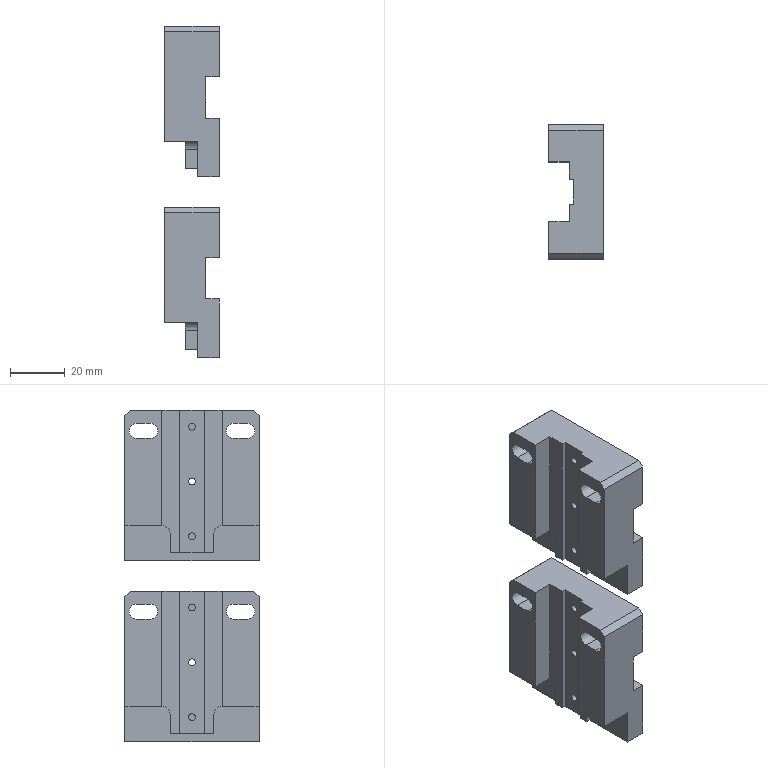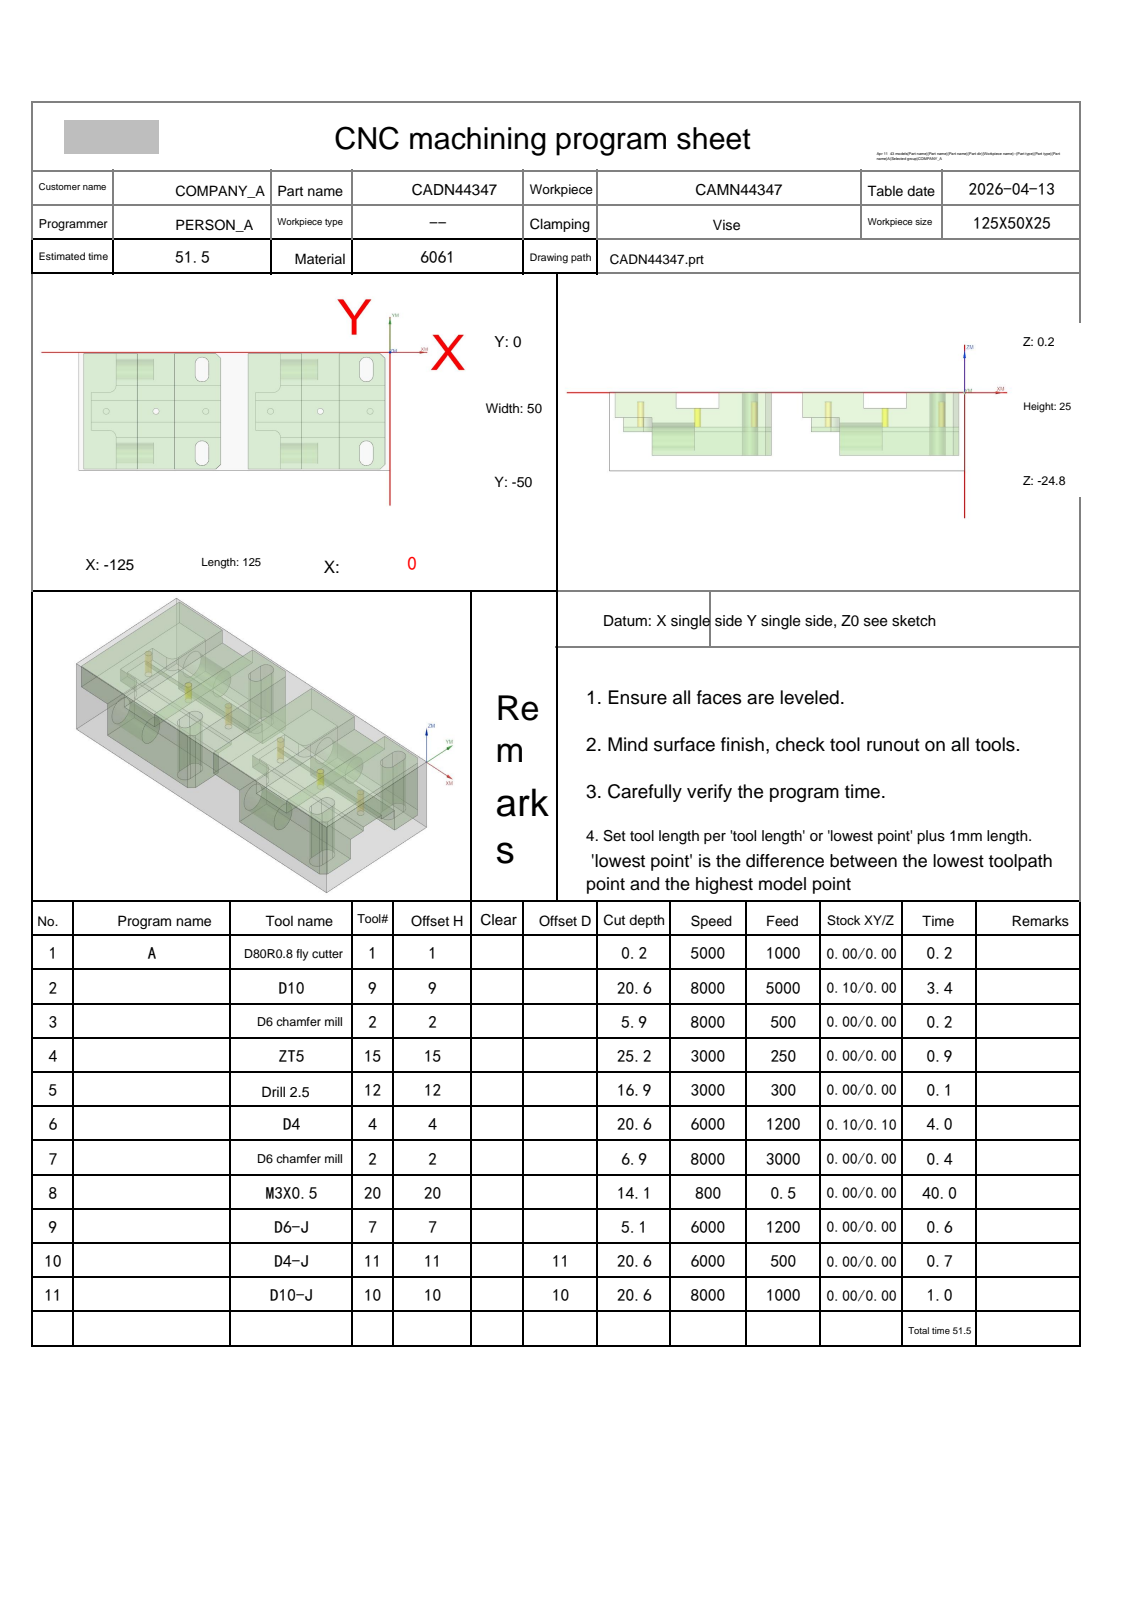NC program | NX | posted by the shop | part box 19.9 x 49 x 121 mm
Lines 1033 to 1849 of 3925:
N6 T04 M06
(D4  D=4. R=0. H=04 ce=0.10 di=0.10)
G00 G90 G54 X-10.15 Y-42.75 M03 S6000
G43 H04 Z20.
M08
Z.5
G01 Y-45.25 Z.456 F1200.
G03 X-9.5 Y-45.9 Z.438 I.65 J0.0
X-8.85 Y-45.25 Z.42 I0.0 J.65
G01 Y-40.25 Z.331
G03 X-9.5 Y-39.6 Z.313 I-.65 J0.0
X-10.15 Y-40.25 Z.295 I0.0 J-.65
G01 Y-45.25 Z.207
G03 X-9.5 Y-45.9 Z.189 I.65 J0.0
X-8.85 Y-45.25 Z.171 I0.0 J.65
G01 Y-40.25 Z.083
G03 X-9.5 Y-39.6 Z.065 I-.65 J0.0
X-10.15 Y-40.25 Z.047 I0.0 J-.65
G01 Y-45.25 Z-.042
G03 X-9.5 Y-45.9 Z-.06 I.65 J0.0
X-8.85 Y-45.25 Z-.078 I0.0 J.65
G01 Y-40.25 Z-.166
G03 X-9.5 Y-39.6 Z-.184 I-.65 J0.0
X-10.15 Y-40.25 Z-.202 I0.0 J-.65
G01 Y-45.25 Z-.291
G03 X-9.5 Y-45.9 Z-.309 I.65 J0.0
X-8.85 Y-45.25 Z-.327 I0.0 J.65
G01 Y-40.25 Z-.415
G03 X-9.5 Y-39.6 Z-.433 I-.65 J0.0
X-10.15 Y-40.25 Z-.451 I0.0 J-.65
G01 Y-45.25 Z-.539
G03 X-9.5 Y-45.9 Z-.557 I.65 J0.0
X-8.85 Y-45.25 Z-.575 I0.0 J.65
G01 Y-40.25 Z-.664
G03 X-9.5 Y-39.6 Z-.682 I-.65 J0.0
X-10.15 Y-40.25 Z-.7 I0.0 J-.65
G01 Y-45.25 Z-.788
G03 X-9.5 Y-45.9 Z-.806 I.65 J0.0
X-8.85 Y-45.25 Z-.824 I0.0 J.65
G01 Y-40.25 Z-.913
G03 X-9.5 Y-39.6 Z-.931 I-.65 J0.0
X-10.15 Y-40.25 Z-.949 I0.0 J-.65
G01 Y-45.25 Z-1.037
G03 X-9.5 Y-45.9 Z-1.055 I.65 J0.0
X-8.85 Y-45.25 Z-1.073 I0.0 J.65
G01 Y-40.25 Z-1.161
G03 X-9.5 Y-39.6 Z-1.179 I-.65 J0.0
X-10.15 Y-40.25 Z-1.198 I0.0 J-.65
G01 Y-45.25 Z-1.286
G03 X-9.5 Y-45.9 Z-1.304 I.65 J0.0
X-8.85 Y-45.25 Z-1.322 I0.0 J.65
G01 Y-40.25 Z-1.41
G03 X-9.5 Y-39.6 Z-1.428 I-.65 J0.0
X-10.15 Y-40.25 Z-1.446 I0.0 J-.65
G01 Y-45.25 Z-1.535
G03 X-9.5 Y-45.9 Z-1.553 I.65 J0.0
X-8.85 Y-45.25 Z-1.571 I0.0 J.65
G01 Y-40.25 Z-1.659
G03 X-9.5 Y-39.6 Z-1.677 I-.65 J0.0
X-10.15 Y-40.25 Z-1.695 I0.0 J-.65
G01 Y-45.25 Z-1.783
G03 X-9.5 Y-45.9 Z-1.801 I.65 J0.0
X-8.85 Y-45.25 Z-1.82 I0.0 J.65
G01 Y-40.25 Z-1.908
G03 X-9.5 Y-39.6 Z-1.926 I-.65 J0.0
X-10.15 Y-40.25 Z-1.944 I0.0 J-.65
G01 Y-45.25 Z-2.032
G03 X-9.5 Y-45.9 Z-2.05 I.65 J0.0
X-8.85 Y-45.25 Z-2.068 I0.0 J.65
G01 Y-40.25 Z-2.157
G03 X-9.5 Y-39.6 Z-2.175 I-.65 J0.0
X-10.15 Y-40.25 Z-2.193 I0.0 J-.65
G01 Y-45.25 Z-2.281
G03 X-9.5 Y-45.9 Z-2.299 I.65 J0.0
X-8.85 Y-45.25 Z-2.317 I0.0 J.65
G01 Y-40.25 Z-2.405
G03 X-9.5 Y-39.6 Z-2.424 I-.65 J0.0
X-10.15 Y-40.25 Z-2.442 I0.0 J-.65
G01 Y-45.25 Z-2.53
G03 X-9.5 Y-45.9 Z-2.548 I.65 J0.0
X-8.85 Y-45.25 Z-2.566 I0.0 J.65
G01 Y-40.25 Z-2.654
G03 X-9.5 Y-39.6 Z-2.672 I-.65 J0.0
X-10.15 Y-40.25 Z-2.69 I0.0 J-.65
G01 Y-45.25 Z-2.779
G03 X-9.5 Y-45.9 Z-2.797 I.65 J0.0
X-8.85 Y-45.25 Z-2.815 I0.0 J.65
G01 Y-40.25 Z-2.903
G03 X-9.5 Y-39.6 Z-2.921 I-.65 J0.0
X-10.15 Y-40.25 Z-2.939 I0.0 J-.65
G01 Y-45.25 Z-3.027
G03 X-9.5 Y-45.9 Z-3.046 I.65 J0.0
X-8.85 Y-45.25 Z-3.064 I0.0 J.65
G01 Y-40.25 Z-3.152
G03 X-9.5 Y-39.6 Z-3.17 I-.65 J0.0
X-10.15 Y-40.25 Z-3.188 I0.0 J-.65
G01 Y-45.25 Z-3.276
G03 X-9.5 Y-45.9 Z-3.294 I.65 J0.0
X-8.85 Y-45.25 Z-3.312 I0.0 J.65
G01 Y-40.25 Z-3.401
G03 X-9.5 Y-39.6 Z-3.419 I-.65 J0.0
X-10.15 Y-40.25 Z-3.437 I0.0 J-.65
G01 Y-45.25 Z-3.525
G03 X-9.5 Y-45.9 Z-3.543 I.65 J0.0
X-8.85 Y-45.25 Z-3.561 I0.0 J.65
G01 Y-40.25 Z-3.65
G03 X-9.5 Y-39.6 Z-3.668 I-.65 J0.0
X-10.15 Y-40.25 Z-3.686 I0.0 J-.65
G01 Y-45.25 Z-3.774
G03 X-9.5 Y-45.9 Z-3.792 I.65 J0.0
X-8.85 Y-45.25 Z-3.81 I0.0 J.65
G01 Y-40.25 Z-3.898
G03 X-9.5 Y-39.6 Z-3.916 I-.65 J0.0
X-10.15 Y-40.25 Z-3.934 I0.0 J-.65
G01 Y-45.25 Z-4.023
G03 X-9.5 Y-45.9 Z-4.041 I.65 J0.0
X-8.85 Y-45.25 Z-4.059 I0.0 J.65
G01 Y-40.25 Z-4.147
G03 X-9.5 Y-39.6 Z-4.165 I-.65 J0.0
X-10.15 Y-40.25 Z-4.183 I0.0 J-.65
G01 Y-45.25 Z-4.272
G03 X-9.5 Y-45.9 Z-4.29 I.65 J0.0
X-8.85 Y-45.25 Z-4.308 I0.0 J.65
G01 Y-40.25 Z-4.396
G03 X-9.5 Y-39.6 Z-4.414 I-.65 J0.0
X-10.15 Y-40.25 Z-4.432 I0.0 J-.65
G01 Y-45.25 Z-4.52
G03 X-9.5 Y-45.9 Z-4.538 I.65 J0.0
X-8.85 Y-45.25 Z-4.556 I0.0 J.65
G01 Y-40.25 Z-4.645
G03 X-9.5 Y-39.6 Z-4.663 I-.65 J0.0
X-10.15 Y-40.25 Z-4.681 I0.0 J-.65
G01 Y-45.25 Z-4.769
G03 X-9.5 Y-45.9 Z-4.787 I.65 J0.0
X-8.85 Y-45.25 Z-4.805 I0.0 J.65
G01 Y-40.25 Z-4.894
G03 X-9.5 Y-39.6 Z-4.912 I-.65 J0.0
X-10.15 Y-40.25 Z-4.93 I0.0 J-.65
G01 Y-45.25 Z-5.018
G03 X-9.5 Y-45.9 Z-5.036 I.65 J0.0
X-8.85 Y-45.25 Z-5.054 I0.0 J.65
G01 Y-40.25 Z-5.142
G03 X-9.5 Y-39.6 Z-5.16 I-.65 J0.0
X-10.15 Y-40.25 Z-5.178 I0.0 J-.65
G01 Y-45.25 Z-5.267
G03 X-9.5 Y-45.9 Z-5.285 I.65 J0.0
X-8.85 Y-45.25 Z-5.303 I0.0 J.65
G01 Y-40.25 Z-5.391
G03 X-9.5 Y-39.6 Z-5.409 I-.65 J0.0
X-10.15 Y-40.25 Z-5.427 I0.0 J-.65
G01 Y-45.25 Z-5.516
G03 X-9.5 Y-45.9 Z-5.534 I.65 J0.0
X-8.85 Y-45.25 Z-5.552 I0.0 J.65
G01 Y-40.25 Z-5.64
G03 X-9.5 Y-39.6 Z-5.658 I-.65 J0.0
X-10.15 Y-40.25 Z-5.676 I0.0 J-.65
G01 Y-45.25 Z-5.764
G03 X-9.5 Y-45.9 Z-5.782 I.65 J0.0
X-8.85 Y-45.25 Z-5.8 I0.0 J.65
G01 Y-40.25 Z-5.889
G03 X-9.5 Y-39.6 Z-5.907 I-.65 J0.0
X-10.15 Y-40.25 Z-5.925 I0.0 J-.65
G01 Y-45.25 Z-6.013
G03 X-9.5 Y-45.9 Z-6.031 I.65 J0.0
X-8.85 Y-45.25 Z-6.049 I0.0 J.65
G01 Y-40.25 Z-6.138
G03 X-9.5 Y-39.6 Z-6.156 I-.65 J0.0
X-10.15 Y-40.25 Z-6.174 I0.0 J-.65
G01 Y-45.25 Z-6.262
G03 X-9.5 Y-45.9 Z-6.28 I.65 J0.0
X-8.85 Y-45.25 Z-6.298 I0.0 J.65
G01 Y-40.25 Z-6.386
G03 X-9.5 Y-39.6 Z-6.404 I-.65 J0.0
X-10.15 Y-40.25 Z-6.423 I0.0 J-.65
G01 Y-45.25 Z-6.511
G03 X-9.5 Y-45.9 Z-6.529 I.65 J0.0
X-8.85 Y-45.25 Z-6.547 I0.0 J.65
G01 Y-40.25 Z-6.635
G03 X-9.5 Y-39.6 Z-6.653 I-.65 J0.0
X-10.15 Y-40.25 Z-6.671 I0.0 J-.65
G01 Y-45.25 Z-6.76
G03 X-9.5 Y-45.9 Z-6.778 I.65 J0.0
X-8.85 Y-45.25 Z-6.796 I0.0 J.65
G01 Y-40.25 Z-6.884
G03 X-9.5 Y-39.6 Z-6.902 I-.65 J0.0
X-10.15 Y-40.25 Z-6.92 I0.0 J-.65
G01 Y-45.25 Z-7.008
G03 X-9.5 Y-45.9 Z-7.026 I.65 J0.0
X-8.85 Y-45.25 Z-7.045 I0.0 J.65
G01 Y-40.25 Z-7.133
G03 X-9.5 Y-39.6 Z-7.151 I-.65 J0.0
X-10.15 Y-40.25 Z-7.169 I0.0 J-.65
G01 Y-45.25 Z-7.257
G03 X-9.5 Y-45.9 Z-7.275 I.65 J0.0
X-8.85 Y-45.25 Z-7.293 I0.0 J.65
G01 Y-40.25 Z-7.382
G03 X-9.5 Y-39.6 Z-7.4 I-.65 J0.0
X-10.15 Y-40.25 Z-7.418 I0.0 J-.65
G01 Y-45.25 Z-7.506
G03 X-9.5 Y-45.9 Z-7.524 I.65 J0.0
X-8.85 Y-45.25 Z-7.542 I0.0 J.65
G01 Y-40.25 Z-7.63
G03 X-9.5 Y-39.6 Z-7.649 I-.65 J0.0
X-10.15 Y-40.25 Z-7.667 I0.0 J-.65
G01 Y-45.25 Z-7.755
G03 X-9.5 Y-45.9 Z-7.773 I.65 J0.0
X-8.85 Y-45.25 Z-7.791 I0.0 J.65
G01 Y-40.25 Z-7.879
G03 X-9.5 Y-39.6 Z-7.897 I-.65 J0.0
X-10.15 Y-40.25 Z-7.915 I0.0 J-.65
G01 Y-45.25 Z-8.004
G03 X-9.5 Y-45.9 Z-8.022 I.65 J0.0
X-8.85 Y-45.25 Z-8.04 I0.0 J.65
G01 Y-40.25 Z-8.128
G03 X-9.5 Y-39.6 Z-8.146 I-.65 J0.0
X-10.15 Y-40.25 Z-8.164 I0.0 J-.65
G01 Y-45.25 Z-8.252
G03 X-9.5 Y-45.9 Z-8.271 I.65 J0.0
X-8.85 Y-45.25 Z-8.289 I0.0 J.65
G01 Y-40.25 Z-8.377
G03 X-9.5 Y-39.6 Z-8.395 I-.65 J0.0
X-10.15 Y-40.25 Z-8.413 I0.0 J-.65
G01 Y-45.25 Z-8.501
G03 X-9.5 Y-45.9 Z-8.519 I.65 J0.0
X-8.85 Y-45.25 Z-8.537 I0.0 J.65
G01 Y-40.25 Z-8.626
G03 X-9.5 Y-39.6 Z-8.644 I-.65 J0.0
X-10.15 Y-40.25 Z-8.662 I0.0 J-.65
G01 Y-45.25 Z-8.75
G03 X-9.5 Y-45.9 Z-8.768 I.65 J0.0
X-8.85 Y-45.25 Z-8.786 I0.0 J.65
G01 Y-40.25 Z-8.875
G03 X-9.5 Y-39.6 Z-8.893 I-.65 J0.0
X-10.15 Y-40.25 Z-8.911 I0.0 J-.65
G01 Y-45.25 Z-8.999
G03 X-9.5 Y-45.9 Z-9.017 I.65 J0.0
X-8.85 Y-45.25 Z-9.035 I0.0 J.65
G01 Y-40.25 Z-9.123
G03 X-9.5 Y-39.6 Z-9.141 I-.65 J0.0
X-10.15 Y-40.25 Z-9.159 I0.0 J-.65
G01 Y-45.25 Z-9.248
G03 X-9.5 Y-45.9 Z-9.266 I.65 J0.0
X-8.85 Y-45.25 Z-9.284 I0.0 J.65
G01 Y-40.25 Z-9.372
G03 X-9.5 Y-39.6 Z-9.39 I-.65 J0.0
X-10.15 Y-40.25 Z-9.408 I0.0 J-.65
G01 Y-45.25 Z-9.497
G03 X-9.5 Y-45.9 Z-9.515 I.65 J0.0
X-8.85 Y-45.25 Z-9.533 I0.0 J.65
G01 Y-40.25 Z-9.621
G03 X-9.5 Y-39.6 Z-9.639 I-.65 J0.0
X-10.15 Y-40.25 Z-9.657 I0.0 J-.65
G01 Y-45.25 Z-9.745
G03 X-9.5 Y-45.9 Z-9.763 I.65 J0.0
X-8.85 Y-45.25 Z-9.781 I0.0 J.65
G01 Y-40.25 Z-9.87
G03 X-9.5 Y-39.6 Z-9.888 I-.65 J0.0
X-10.15 Y-40.25 Z-9.906 I0.0 J-.65
G01 Y-45.25 Z-9.994
G03 X-9.5 Y-45.9 Z-10.012 I.65 J0.0
X-8.85 Y-45.25 Z-10.03 I0.0 J.65
G01 Y-40.25 Z-10.119
G03 X-9.5 Y-39.6 Z-10.137 I-.65 J0.0
X-10.15 Y-40.25 Z-10.155 I0.0 J-.65
G01 Y-45.25 Z-10.243
G03 X-9.5 Y-45.9 Z-10.261 I.65 J0.0
X-8.85 Y-45.25 Z-10.279 I0.0 J.65
G01 Y-40.25 Z-10.367
G03 X-9.5 Y-39.6 Z-10.385 I-.65 J0.0
X-10.15 Y-40.25 Z-10.403 I0.0 J-.65
G01 Y-45.25 Z-10.492
G03 X-9.5 Y-45.9 Z-10.51 I.65 J0.0
X-8.85 Y-45.25 Z-10.528 I0.0 J.65
G01 Y-40.25 Z-10.616
G03 X-9.5 Y-39.6 Z-10.634 I-.65 J0.0
X-10.15 Y-40.25 Z-10.652 I0.0 J-.65
G01 Y-45.25 Z-10.741
G03 X-9.5 Y-45.9 Z-10.759 I.65 J0.0
X-8.85 Y-45.25 Z-10.777 I0.0 J.65
G01 Y-40.25 Z-10.865
G03 X-9.5 Y-39.6 Z-10.883 I-.65 J0.0
X-10.15 Y-40.25 Z-10.901 I0.0 J-.65
G01 Y-45.25 Z-10.989
G03 X-9.5 Y-45.9 Z-11.007 I.65 J0.0
X-8.85 Y-45.25 Z-11.025 I0.0 J.65
G01 Y-40.25 Z-11.114
G03 X-9.5 Y-39.6 Z-11.132 I-.65 J0.0
X-10.15 Y-40.25 Z-11.15 I0.0 J-.65
G01 Y-45.25 Z-11.238
G03 X-9.5 Y-45.9 Z-11.256 I.65 J0.0
X-8.85 Y-45.25 Z-11.274 I0.0 J.65
G01 Y-40.25 Z-11.363
G03 X-9.5 Y-39.6 Z-11.381 I-.65 J0.0
X-10.15 Y-40.25 Z-11.399 I0.0 J-.65
G01 Y-45.25 Z-11.487
G03 X-9.5 Y-45.9 Z-11.505 I.65 J0.0
X-8.85 Y-45.25 Z-11.523 I0.0 J.65
G01 Y-40.25 Z-11.611
G03 X-9.5 Y-39.6 Z-11.629 I-.65 J0.0
X-10.15 Y-40.25 Z-11.648 I0.0 J-.65
G01 Y-45.25 Z-11.736
G03 X-9.5 Y-45.9 Z-11.754 I.65 J0.0
X-8.85 Y-45.25 Z-11.772 I0.0 J.65
G01 Y-40.25 Z-11.86
G03 X-9.5 Y-39.6 Z-11.878 I-.65 J0.0
X-10.15 Y-40.25 Z-11.896 I0.0 J-.65
G01 Y-45.25 Z-11.985
G03 X-9.5 Y-45.9 Z-12.003 I.65 J0.0
X-8.85 Y-45.25 Z-12.021 I0.0 J.65
G01 Y-40.25 Z-12.109
G03 X-9.5 Y-39.6 Z-12.127 I-.65 J0.0
X-10.15 Y-40.25 Z-12.145 I0.0 J-.65
G01 Y-45.25 Z-12.233
G03 X-9.5 Y-45.9 Z-12.251 I.65 J0.0
X-8.85 Y-45.25 Z-12.27 I0.0 J.65
G01 Y-40.25 Z-12.358
G03 X-9.5 Y-39.6 Z-12.376 I-.65 J0.0
X-10.15 Y-40.25 Z-12.394 I0.0 J-.65
G01 Y-45.25 Z-12.482
G03 X-9.5 Y-45.9 Z-12.5 I.65 J0.0
X-8.85 Y-45.25 Z-12.518 I0.0 J.65
G01 Y-40.25 Z-12.607
G03 X-9.5 Y-39.6 Z-12.625 I-.65 J0.0
X-10.15 Y-40.25 Z-12.643 I0.0 J-.65
G01 Y-45.25 Z-12.731
G03 X-9.5 Y-45.9 Z-12.749 I.65 J0.0
X-8.85 Y-45.25 Z-12.767 I0.0 J.65
G01 Y-40.25 Z-12.855
G03 X-9.5 Y-39.6 Z-12.874 I-.65 J0.0
X-10.15 Y-40.25 Z-12.892 I0.0 J-.65
G01 Y-45.25 Z-12.98
G03 X-9.5 Y-45.9 Z-12.998 I.65 J0.0
X-8.85 Y-45.25 Z-13.016 I0.0 J.65
G01 Y-40.25 Z-13.104
G03 X-9.5 Y-39.6 Z-13.122 I-.65 J0.0
X-10.15 Y-40.25 Z-13.14 I0.0 J-.65
G01 Y-45.25 Z-13.229
G03 X-9.5 Y-45.9 Z-13.247 I.65 J0.0
X-8.85 Y-45.25 Z-13.265 I0.0 J.65
G01 Y-40.25 Z-13.353
G03 X-9.5 Y-39.6 Z-13.371 I-.65 J0.0
X-10.15 Y-40.25 Z-13.389 I0.0 J-.65
G01 Y-45.25 Z-13.477
G03 X-9.5 Y-45.9 Z-13.496 I.65 J0.0
X-8.85 Y-45.25 Z-13.514 I0.0 J.65
G01 Y-40.25 Z-13.602
G03 X-9.5 Y-39.6 Z-13.62 I-.65 J0.0
X-10.15 Y-40.25 Z-13.638 I0.0 J-.65
G01 Y-45.25 Z-13.726
G03 X-9.5 Y-45.9 Z-13.744 I.65 J0.0
X-8.85 Y-45.25 Z-13.762 I0.0 J.65
G01 Y-40.25 Z-13.851
G03 X-9.5 Y-39.6 Z-13.869 I-.65 J0.0
X-10.15 Y-40.25 Z-13.887 I0.0 J-.65
G01 Y-45.25 Z-13.975
G03 X-9.5 Y-45.9 Z-13.993 I.65 J0.0
X-8.85 Y-45.25 Z-14.011 I0.0 J.65
G01 Y-40.25 Z-14.1
G03 X-9.5 Y-39.6 Z-14.118 I-.65 J0.0
X-10.15 Y-40.25 Z-14.136 I0.0 J-.65
G01 Y-45.25 Z-14.224
G03 X-9.5 Y-45.9 Z-14.242 I.65 J0.0
X-8.85 Y-45.25 Z-14.26 I0.0 J.65
G01 Y-40.25 Z-14.348
G03 X-9.5 Y-39.6 Z-14.366 I-.65 J0.0
X-10.15 Y-40.25 Z-14.384 I0.0 J-.65
G01 Y-45.25 Z-14.473
G03 X-9.5 Y-45.9 Z-14.491 I.65 J0.0
X-8.85 Y-45.25 Z-14.509 I0.0 J.65
G01 Y-40.25 Z-14.597
G03 X-9.5 Y-39.6 Z-14.615 I-.65 J0.0
X-10.15 Y-40.25 Z-14.633 I0.0 J-.65
G01 Y-45.25 Z-14.722
G03 X-9.5 Y-45.9 Z-14.74 I.65 J0.0
X-8.85 Y-45.25 Z-14.758 I0.0 J.65
G01 Y-40.25 Z-14.846
G03 X-9.5 Y-39.6 Z-14.864 I-.65 J0.0
X-10.15 Y-40.25 Z-14.882 I0.0 J-.65
G01 Y-45.25 Z-14.97
G03 X-9.5 Y-45.9 Z-14.988 I.65 J0.0
X-8.85 Y-45.25 Z-15.006 I0.0 J.65
G01 Y-40.25 Z-15.095
G03 X-9.5 Y-39.6 Z-15.113 I-.65 J0.0
X-10.15 Y-40.25 Z-15.131 I0.0 J-.65
G01 Y-45.25 Z-15.219
G03 X-9.5 Y-45.9 Z-15.237 I.65 J0.0
X-8.85 Y-45.25 Z-15.255 I0.0 J.65
G01 Y-40.25 Z-15.344
G03 X-9.5 Y-39.6 Z-15.362 I-.65 J0.0
X-10.15 Y-40.25 Z-15.38 I0.0 J-.65
G01 Y-45.25 Z-15.468
G03 X-9.5 Y-45.9 Z-15.486 I.65 J0.0
X-8.85 Y-45.25 Z-15.504 I0.0 J.65
G01 Y-40.25 Z-15.592
G03 X-9.5 Y-39.6 Z-15.61 I-.65 J0.0
X-10.15 Y-40.25 Z-15.628 I0.0 J-.65
G01 Y-45.25 Z-15.717
G03 X-9.5 Y-45.9 Z-15.735 I.65 J0.0
X-8.85 Y-45.25 Z-15.753 I0.0 J.65
G01 Y-40.25 Z-15.841
G03 X-9.5 Y-39.6 Z-15.859 I-.65 J0.0
X-10.15 Y-40.25 Z-15.877 I0.0 J-.65
G01 Y-45.25 Z-15.966
G03 X-9.5 Y-45.9 Z-15.984 I.65 J0.0
X-8.85 Y-45.25 Z-16.002 I0.0 J.65
G01 Y-40.25 Z-16.09
G03 X-9.5 Y-39.6 Z-16.108 I-.65 J0.0
X-10.15 Y-40.25 Z-16.126 I0.0 J-.65
G01 Y-45.25 Z-16.214
G03 X-9.5 Y-45.9 Z-16.232 I.65 J0.0
X-8.85 Y-45.25 Z-16.25 I0.0 J.65
G01 Y-40.25 Z-16.339
G03 X-9.5 Y-39.6 Z-16.357 I-.65 J0.0
X-10.15 Y-40.25 Z-16.375 I0.0 J-.65
G01 Y-45.25 Z-16.463
G03 X-9.5 Y-45.9 Z-16.481 I.65 J0.0
X-8.85 Y-45.25 Z-16.499 I0.0 J.65
G01 Y-40.25 Z-16.588
G03 X-9.5 Y-39.6 Z-16.606 I-.65 J0.0
X-10.15 Y-40.25 Z-16.624 I0.0 J-.65
G01 Y-45.25 Z-16.712
G03 X-9.5 Y-45.9 Z-16.73 I.65 J0.0
X-8.85 Y-45.25 Z-16.748 I0.0 J.65
G01 Y-40.25 Z-16.836
G03 X-9.5 Y-39.6 Z-16.854 I-.65 J0.0
X-10.15 Y-40.25 Z-16.873 I0.0 J-.65
G01 Y-45.25 Z-16.961
G03 X-9.5 Y-45.9 Z-16.979 I.65 J0.0
X-8.85 Y-45.25 Z-16.997 I0.0 J.65
G01 Y-40.25 Z-17.085
G03 X-9.5 Y-39.6 Z-17.103 I-.65 J0.0
X-10.15 Y-40.25 Z-17.121 I0.0 J-.65
G01 Y-45.25 Z-17.21
G03 X-9.5 Y-45.9 Z-17.228 I.65 J0.0
X-8.85 Y-45.25 Z-17.246 I0.0 J.65
G01 Y-40.25 Z-17.334
G03 X-9.5 Y-39.6 Z-17.352 I-.65 J0.0
X-10.15 Y-40.25 Z-17.37 I0.0 J-.65
G01 Y-45.25 Z-17.458
G03 X-9.5 Y-45.9 Z-17.476 I.65 J0.0
X-8.85 Y-45.25 Z-17.495 I0.0 J.65
G01 Y-40.25 Z-17.583
G03 X-9.5 Y-39.6 Z-17.601 I-.65 J0.0
X-10.15 Y-40.25 Z-17.619 I0.0 J-.65
G01 Y-45.25 Z-17.707
G03 X-9.5 Y-45.9 Z-17.725 I.65 J0.0
X-8.85 Y-45.25 Z-17.743 I0.0 J.65
G01 Y-40.25 Z-17.832
G03 X-9.5 Y-39.6 Z-17.85 I-.65 J0.0
X-10.15 Y-40.25 Z-17.868 I0.0 J-.65
G01 Y-45.25 Z-17.956
G03 X-9.5 Y-45.9 Z-17.974 I.65 J0.0
X-8.85 Y-45.25 Z-17.992 I0.0 J.65
G01 Y-40.25 Z-18.08
G03 X-9.5 Y-39.6 Z-18.099 I-.65 J0.0
X-10.15 Y-40.25 Z-18.117 I0.0 J-.65
G01 Y-45.25 Z-18.205
G03 X-9.5 Y-45.9 Z-18.223 I.65 J0.0
X-8.85 Y-45.25 Z-18.241 I0.0 J.65
G01 Y-40.25 Z-18.329
G03 X-9.5 Y-39.6 Z-18.347 I-.65 J0.0
X-10.15 Y-40.25 Z-18.365 I0.0 J-.65
G01 Y-45.25 Z-18.454
G03 X-9.5 Y-45.9 Z-18.472 I.65 J0.0
X-8.85 Y-45.25 Z-18.49 I0.0 J.65
G01 Y-40.25 Z-18.578
G03 X-9.5 Y-39.6 Z-18.596 I-.65 J0.0
X-10.15 Y-40.25 Z-18.614 I0.0 J-.65
G01 Y-45.25 Z-18.702
G03 X-9.5 Y-45.9 Z-18.721 I.65 J0.0
X-8.85 Y-45.25 Z-18.739 I0.0 J.65
G01 Y-40.25 Z-18.827
G03 X-9.5 Y-39.6 Z-18.845 I-.65 J0.0
X-10.15 Y-40.25 Z-18.863 I0.0 J-.65
G01 Y-45.25 Z-18.951
G03 X-9.5 Y-45.9 Z-18.969 I.65 J0.0
X-8.85 Y-45.25 Z-18.987 I0.0 J.65
G01 Y-40.25 Z-19.076
G03 X-9.5 Y-39.6 Z-19.094 I-.65 J0.0
X-10.15 Y-40.25 Z-19.112 I0.0 J-.65
G01 Y-45.25 Z-19.2
G03 X-9.5 Y-45.9 Z-19.218 I.65 J0.0
X-8.85 Y-45.25 Z-19.236 I0.0 J.65
G01 Y-40.25 Z-19.325
G03 X-9.5 Y-39.6 Z-19.343 I-.65 J0.0
X-10.15 Y-40.25 Z-19.361 I0.0 J-.65
G01 Y-45.25 Z-19.449
G03 X-9.5 Y-45.9 Z-19.467 I.65 J0.0
X-8.85 Y-45.25 Z-19.485 I0.0 J.65
G01 Y-40.25 Z-19.573
G03 X-9.5 Y-39.6 Z-19.591 I-.65 J0.0
X-10.15 Y-40.25 Z-19.609 I0.0 J-.65
G01 Y-45.25 Z-19.698
G03 X-9.5 Y-45.9 Z-19.716 I.65 J0.0
X-8.85 Y-45.25 Z-19.734 I0.0 J.65
G01 Y-40.25 Z-19.822
G03 X-9.5 Y-39.6 Z-19.84 I-.65 J0.0
X-10.15 Y-40.25 Z-19.858 I0.0 J-.65
G01 Y-45.25 Z-19.947
G03 X-9.5 Y-45.9 Z-19.965 I.65 J0.0
X-8.85 Y-45.25 Z-19.983 I0.0 J.65
G01 Y-40.25 Z-20.071
G03 X-9.5 Y-39.6 Z-20.089 I-.65 J0.0
X-10.15 Y-40.25 Z-20.107 I0.0 J-.65
G01 Y-45.25 Z-20.195
G03 X-9.5 Y-45.9 Z-20.213 I.65 J0.0
X-8.85 Y-45.25 Z-20.231 I0.0 J.65
G01 Y-40.25 Z-20.32
G03 X-9.5 Y-39.6 Z-20.338 I-.65 J0.0
X-10.15 Y-40.25 Z-20.356 I0.0 J-.65
G01 Y-42.75 Z-20.4
Y-45.25
G03 X-9.5 Y-45.9 I.65 J0.0
X-8.85 Y-45.25 I0.0 J.65
G01 Y-40.25
G03 X-9.5 Y-39.6 I-.65 J0.0
X-10.15 Y-40.25 I0.0 J-.65
G01 Y-42.75
Y-43.25
Z-19.4
G00 Z20.
X-8.85 Y-7.25
Z.5
G01 Y-4.75 Z.456
G03 X-9.5 Y-4.1 Z.438 I-.65 J0.0
X-10.15 Y-4.75 Z.42 I0.0 J-.65
G01 Y-9.75 Z.331
G03 X-9.5 Y-10.4 Z.313 I.65 J0.0
X-8.85 Y-9.75 Z.295 I0.0 J.65
G01 Y-4.75 Z.207
G03 X-9.5 Y-4.1 Z.189 I-.65 J0.0
X-10.15 Y-4.75 Z.171 I0.0 J-.65
G01 Y-9.75 Z.083
G03 X-9.5 Y-10.4 Z.065 I.65 J0.0
X-8.85 Y-9.75 Z.047 I0.0 J.65
G01 Y-4.75 Z-.042
G03 X-9.5 Y-4.1 Z-.06 I-.65 J0.0
X-10.15 Y-4.75 Z-.078 I0.0 J-.65
G01 Y-9.75 Z-.166
G03 X-9.5 Y-10.4 Z-.184 I.65 J0.0
X-8.85 Y-9.75 Z-.202 I0.0 J.65
G01 Y-4.75 Z-.291
G03 X-9.5 Y-4.1 Z-.309 I-.65 J0.0
X-10.15 Y-4.75 Z-.327 I0.0 J-.65
G01 Y-9.75 Z-.415
G03 X-9.5 Y-10.4 Z-.433 I.65 J0.0
X-8.85 Y-9.75 Z-.451 I0.0 J.65
G01 Y-4.75 Z-.539
G03 X-9.5 Y-4.1 Z-.557 I-.65 J0.0
X-10.15 Y-4.75 Z-.575 I0.0 J-.65
G01 Y-9.75 Z-.664
G03 X-9.5 Y-10.4 Z-.682 I.65 J0.0
X-8.85 Y-9.75 Z-.7 I0.0 J.65
G01 Y-4.75 Z-.788
G03 X-9.5 Y-4.1 Z-.806 I-.65 J0.0
X-10.15 Y-4.75 Z-.824 I0.0 J-.65
G01 Y-9.75 Z-.913
G03 X-9.5 Y-10.4 Z-.931 I.65 J0.0
X-8.85 Y-9.75 Z-.949 I0.0 J.65
G01 Y-4.75 Z-1.037
G03 X-9.5 Y-4.1 Z-1.055 I-.65 J0.0
X-10.15 Y-4.75 Z-1.073 I0.0 J-.65
G01 Y-9.75 Z-1.161
G03 X-9.5 Y-10.4 Z-1.179 I.65 J0.0
X-8.85 Y-9.75 Z-1.198 I0.0 J.65
G01 Y-4.75 Z-1.286
G03 X-9.5 Y-4.1 Z-1.304 I-.65 J0.0
X-10.15 Y-4.75 Z-1.322 I0.0 J-.65
G01 Y-9.75 Z-1.41
G03 X-9.5 Y-10.4 Z-1.428 I.65 J0.0
X-8.85 Y-9.75 Z-1.446 I0.0 J.65
G01 Y-4.75 Z-1.535
G03 X-9.5 Y-4.1 Z-1.553 I-.65 J0.0
X-10.15 Y-4.75 Z-1.571 I0.0 J-.65
G01 Y-9.75 Z-1.659
G03 X-9.5 Y-10.4 Z-1.677 I.65 J0.0
X-8.85 Y-9.75 Z-1.695 I0.0 J.65
G01 Y-4.75 Z-1.783
G03 X-9.5 Y-4.1 Z-1.801 I-.65 J0.0
X-10.15 Y-4.75 Z-1.82 I0.0 J-.65
G01 Y-9.75 Z-1.908
G03 X-9.5 Y-10.4 Z-1.926 I.65 J0.0
X-8.85 Y-9.75 Z-1.944 I0.0 J.65
G01 Y-4.75 Z-2.032
G03 X-9.5 Y-4.1 Z-2.05 I-.65 J0.0
X-10.15 Y-4.75 Z-2.068 I0.0 J-.65
G01 Y-9.75 Z-2.157
G03 X-9.5 Y-10.4 Z-2.175 I.65 J0.0
X-8.85 Y-9.75 Z-2.193 I0.0 J.65
G01 Y-4.75 Z-2.281
G03 X-9.5 Y-4.1 Z-2.299 I-.65 J0.0
X-10.15 Y-4.75 Z-2.317 I0.0 J-.65
G01 Y-9.75 Z-2.405
G03 X-9.5 Y-10.4 Z-2.424 I.65 J0.0
X-8.85 Y-9.75 Z-2.442 I0.0 J.65
G01 Y-4.75 Z-2.53
G03 X-9.5 Y-4.1 Z-2.548 I-.65 J0.0
X-10.15 Y-4.75 Z-2.566 I0.0 J-.65
G01 Y-9.75 Z-2.654
G03 X-9.5 Y-10.4 Z-2.672 I.65 J0.0
X-8.85 Y-9.75 Z-2.69 I0.0 J.65
G01 Y-4.75 Z-2.779
G03 X-9.5 Y-4.1 Z-2.797 I-.65 J0.0
X-10.15 Y-4.75 Z-2.815 I0.0 J-.65
G01 Y-9.75 Z-2.903
G03 X-9.5 Y-10.4 Z-2.921 I.65 J0.0
X-8.85 Y-9.75 Z-2.939 I0.0 J.65
G01 Y-4.75 Z-3.027
G03 X-9.5 Y-4.1 Z-3.046 I-.65 J0.0
X-10.15 Y-4.75 Z-3.064 I0.0 J-.65
G01 Y-9.75 Z-3.152
G03 X-9.5 Y-10.4 Z-3.17 I.65 J0.0
X-8.85 Y-9.75 Z-3.188 I0.0 J.65
G01 Y-4.75 Z-3.276
G03 X-9.5 Y-4.1 Z-3.294 I-.65 J0.0
X-10.15 Y-4.75 Z-3.312 I0.0 J-.65
G01 Y-9.75 Z-3.401
G03 X-9.5 Y-10.4 Z-3.419 I.65 J0.0
X-8.85 Y-9.75 Z-3.437 I0.0 J.65
G01 Y-4.75 Z-3.525
G03 X-9.5 Y-4.1 Z-3.543 I-.65 J0.0
X-10.15 Y-4.75 Z-3.561 I0.0 J-.65
G01 Y-9.75 Z-3.65
G03 X-9.5 Y-10.4 Z-3.668 I.65 J0.0
X-8.85 Y-9.75 Z-3.686 I0.0 J.65
G01 Y-4.75 Z-3.774
G03 X-9.5 Y-4.1 Z-3.792 I-.65 J0.0
X-10.15 Y-4.75 Z-3.81 I0.0 J-.65
G01 Y-9.75 Z-3.898
G03 X-9.5 Y-10.4 Z-3.916 I.65 J0.0
X-8.85 Y-9.75 Z-3.934 I0.0 J.65
G01 Y-4.75 Z-4.023
G03 X-9.5 Y-4.1 Z-4.041 I-.65 J0.0
X-10.15 Y-4.75 Z-4.059 I0.0 J-.65
G01 Y-9.75 Z-4.147
G03 X-9.5 Y-10.4 Z-4.165 I.65 J0.0
X-8.85 Y-9.75 Z-4.183 I0.0 J.65
G01 Y-4.75 Z-4.272
G03 X-9.5 Y-4.1 Z-4.29 I-.65 J0.0
X-10.15 Y-4.75 Z-4.308 I0.0 J-.65
G01 Y-9.75 Z-4.396
G03 X-9.5 Y-10.4 Z-4.414 I.65 J0.0
X-8.85 Y-9.75 Z-4.432 I0.0 J.65
G01 Y-4.75 Z-4.52
G03 X-9.5 Y-4.1 Z-4.538 I-.65 J0.0
X-10.15 Y-4.75 Z-4.556 I0.0 J-.65
G01 Y-9.75 Z-4.645
G03 X-9.5 Y-10.4 Z-4.663 I.65 J0.0
X-8.85 Y-9.75 Z-4.681 I0.0 J.65
G01 Y-4.75 Z-4.769
G03 X-9.5 Y-4.1 Z-4.787 I-.65 J0.0
X-10.15 Y-4.75 Z-4.805 I0.0 J-.65
G01 Y-9.75 Z-4.894
G03 X-9.5 Y-10.4 Z-4.912 I.65 J0.0
X-8.85 Y-9.75 Z-4.93 I0.0 J.65
G01 Y-4.75 Z-5.018
G03 X-9.5 Y-4.1 Z-5.036 I-.65 J0.0
X-10.15 Y-4.75 Z-5.054 I0.0 J-.65
G01 Y-9.75 Z-5.142
G03 X-9.5 Y-10.4 Z-5.16 I.65 J0.0
X-8.85 Y-9.75 Z-5.178 I0.0 J.65
G01 Y-4.75 Z-5.267
G03 X-9.5 Y-4.1 Z-5.285 I-.65 J0.0
X-10.15 Y-4.75 Z-5.303 I0.0 J-.65
G01 Y-9.75 Z-5.391
G03 X-9.5 Y-10.4 Z-5.409 I.65 J0.0
X-8.85 Y-9.75 Z-5.427 I0.0 J.65
G01 Y-4.75 Z-5.516
G03 X-9.5 Y-4.1 Z-5.534 I-.65 J0.0
X-10.15 Y-4.75 Z-5.552 I0.0 J-.65
G01 Y-9.75 Z-5.64
G03 X-9.5 Y-10.4 Z-5.658 I.65 J0.0
X-8.85 Y-9.75 Z-5.676 I0.0 J.65
G01 Y-4.75 Z-5.764
G03 X-9.5 Y-4.1 Z-5.782 I-.65 J0.0
X-10.15 Y-4.75 Z-5.8 I0.0 J-.65
G01 Y-9.75 Z-5.889
G03 X-9.5 Y-10.4 Z-5.907 I.65 J0.0
X-8.85 Y-9.75 Z-5.925 I0.0 J.65
G01 Y-4.75 Z-6.013
G03 X-9.5 Y-4.1 Z-6.031 I-.65 J0.0
X-10.15 Y-4.75 Z-6.049 I0.0 J-.65
G01 Y-9.75 Z-6.138
G03 X-9.5 Y-10.4 Z-6.156 I.65 J0.0
X-8.85 Y-9.75 Z-6.174 I0.0 J.65
G01 Y-4.75 Z-6.262
G03 X-9.5 Y-4.1 Z-6.28 I-.65 J0.0
X-10.15 Y-4.75 Z-6.298 I0.0 J-.65
G01 Y-9.75 Z-6.386
G03 X-9.5 Y-10.4 Z-6.404 I.65 J0.0
X-8.85 Y-9.75 Z-6.423 I0.0 J.65
G01 Y-4.75 Z-6.511
G03 X-9.5 Y-4.1 Z-6.529 I-.65 J0.0
X-10.15 Y-4.75 Z-6.547 I0.0 J-.65
G01 Y-9.75 Z-6.635
G03 X-9.5 Y-10.4 Z-6.653 I.65 J0.0
X-8.85 Y-9.75 Z-6.671 I0.0 J.65
G01 Y-4.75 Z-6.76
G03 X-9.5 Y-4.1 Z-6.778 I-.65 J0.0
X-10.15 Y-4.75 Z-6.796 I0.0 J-.65
G01 Y-9.75 Z-6.884
G03 X-9.5 Y-10.4 Z-6.902 I.65 J0.0
X-8.85 Y-9.75 Z-6.92 I0.0 J.65
G01 Y-4.75 Z-7.008
G03 X-9.5 Y-4.1 Z-7.026 I-.65 J0.0
X-10.15 Y-4.75 Z-7.045 I0.0 J-.65
G01 Y-9.75 Z-7.133
G03 X-9.5 Y-10.4 Z-7.151 I.65 J0.0
X-8.85 Y-9.75 Z-7.169 I0.0 J.65
G01 Y-4.75 Z-7.257
G03 X-9.5 Y-4.1 Z-7.275 I-.65 J0.0
X-10.15 Y-4.75 Z-7.293 I0.0 J-.65
G01 Y-9.75 Z-7.382
G03 X-9.5 Y-10.4 Z-7.4 I.65 J0.0
X-8.85 Y-9.75 Z-7.418 I0.0 J.65
G01 Y-4.75 Z-7.506
G03 X-9.5 Y-4.1 Z-7.524 I-.65 J0.0
X-10.15 Y-4.75 Z-7.542 I0.0 J-.65
G01 Y-9.75 Z-7.63
G03 X-9.5 Y-10.4 Z-7.649 I.65 J0.0
X-8.85 Y-9.75 Z-7.667 I0.0 J.65
G01 Y-4.75 Z-7.755
G03 X-9.5 Y-4.1 Z-7.773 I-.65 J0.0
X-10.15 Y-4.75 Z-7.791 I0.0 J-.65
G01 Y-9.75 Z-7.879
G03 X-9.5 Y-10.4 Z-7.897 I.65 J0.0
X-8.85 Y-9.75 Z-7.915 I0.0 J.65
G01 Y-4.75 Z-8.004
G03 X-9.5 Y-4.1 Z-8.022 I-.65 J0.0
X-10.15 Y-4.75 Z-8.04 I0.0 J-.65
G01 Y-9.75 Z-8.128
G03 X-9.5 Y-10.4 Z-8.146 I.65 J0.0
X-8.85 Y-9.75 Z-8.164 I0.0 J.65
G01 Y-4.75 Z-8.252
G03 X-9.5 Y-4.1 Z-8.271 I-.65 J0.0
X-10.15 Y-4.75 Z-8.289 I0.0 J-.65
G01 Y-9.75 Z-8.377
G03 X-9.5 Y-10.4 Z-8.395 I.65 J0.0
X-8.85 Y-9.75 Z-8.413 I0.0 J.65
G01 Y-4.75 Z-8.501
G03 X-9.5 Y-4.1 Z-8.519 I-.65 J0.0
X-10.15 Y-4.75 Z-8.537 I0.0 J-.65
G01 Y-9.75 Z-8.626
G03 X-9.5 Y-10.4 Z-8.644 I.65 J0.0
X-8.85 Y-9.75 Z-8.662 I0.0 J.65
G01 Y-4.75 Z-8.75
G03 X-9.5 Y-4.1 Z-8.768 I-.65 J0.0
X-10.15 Y-4.75 Z-8.786 I0.0 J-.65
G01 Y-9.75 Z-8.875
G03 X-9.5 Y-10.4 Z-8.893 I.65 J0.0
X-8.85 Y-9.75 Z-8.911 I0.0 J.65
G01 Y-4.75 Z-8.999
G03 X-9.5 Y-4.1 Z-9.017 I-.65 J0.0
X-10.15 Y-4.75 Z-9.035 I0.0 J-.65
G01 Y-9.75 Z-9.123
G03 X-9.5 Y-10.4 Z-9.141 I.65 J0.0
X-8.85 Y-9.75 Z-9.159 I0.0 J.65
G01 Y-4.75 Z-9.248
G03 X-9.5 Y-4.1 Z-9.266 I-.65 J0.0
X-10.15 Y-4.75 Z-9.284 I0.0 J-.65
G01 Y-9.75 Z-9.372
G03 X-9.5 Y-10.4 Z-9.39 I.65 J0.0
X-8.85 Y-9.75 Z-9.408 I0.0 J.65
G01 Y-4.75 Z-9.497
G03 X-9.5 Y-4.1 Z-9.515 I-.65 J0.0
X-10.15 Y-4.75 Z-9.533 I0.0 J-.65
G01 Y-9.75 Z-9.621
G03 X-9.5 Y-10.4 Z-9.639 I.65 J0.0
X-8.85 Y-9.75 Z-9.657 I0.0 J.65
G01 Y-4.75 Z-9.745
G03 X-9.5 Y-4.1 Z-9.763 I-.65 J0.0
X-10.15 Y-4.75 Z-9.781 I0.0 J-.65
G01 Y-9.75 Z-9.87
G03 X-9.5 Y-10.4 Z-9.888 I.65 J0.0
X-8.85 Y-9.75 Z-9.906 I0.0 J.65
G01 Y-4.75 Z-9.994
G03 X-9.5 Y-4.1 Z-10.012 I-.65 J0.0
X-10.15 Y-4.75 Z-10.03 I0.0 J-.65
G01 Y-9.75 Z-10.119
G03 X-9.5 Y-10.4 Z-10.137 I.65 J0.0
X-8.85 Y-9.75 Z-10.155 I0.0 J.65
G01 Y-4.75 Z-10.243
G03 X-9.5 Y-4.1 Z-10.261 I-.65 J0.0
X-10.15 Y-4.75 Z-10.279 I0.0 J-.65
G01 Y-9.75 Z-10.367
G03 X-9.5 Y-10.4 Z-10.385 I.65 J0.0
X-8.85 Y-9.75 Z-10.403 I0.0 J.65
G01 Y-4.75 Z-10.492
G03 X-9.5 Y-4.1 Z-10.51 I-.65 J0.0
X-10.15 Y-4.75 Z-10.528 I0.0 J-.65
G01 Y-9.75 Z-10.616
G03 X-9.5 Y-10.4 Z-10.634 I.65 J0.0
X-8.85 Y-9.75 Z-10.652 I0.0 J.65
G01 Y-4.75 Z-10.741
G03 X-9.5 Y-4.1 Z-10.759 I-.65 J0.0
X-10.15 Y-4.75 Z-10.777 I0.0 J-.65
G01 Y-9.75 Z-10.865
G03 X-9.5 Y-10.4 Z-10.883 I.65 J0.0
X-8.85 Y-9.75 Z-10.901 I0.0 J.65
G01 Y-4.75 Z-10.989
G03 X-9.5 Y-4.1 Z-11.007 I-.65 J0.0
X-10.15 Y-4.75 Z-11.025 I0.0 J-.65
G01 Y-9.75 Z-11.114
G03 X-9.5 Y-10.4 Z-11.132 I.65 J0.0
X-8.85 Y-9.75 Z-11.15 I0.0 J.65
G01 Y-4.75 Z-11.238
G03 X-9.5 Y-4.1 Z-11.256 I-.65 J0.0
X-10.15 Y-4.75 Z-11.274 I0.0 J-.65
G01 Y-9.75 Z-11.363
G03 X-9.5 Y-10.4 Z-11.381 I.65 J0.0
X-8.85 Y-9.75 Z-11.399 I0.0 J.65
G01 Y-4.75 Z-11.487
G03 X-9.5 Y-4.1 Z-11.505 I-.65 J0.0
X-10.15 Y-4.75 Z-11.523 I0.0 J-.65
G01 Y-9.75 Z-11.611
G03 X-9.5 Y-10.4 Z-11.629 I.65 J0.0
X-8.85 Y-9.75 Z-11.648 I0.0 J.65